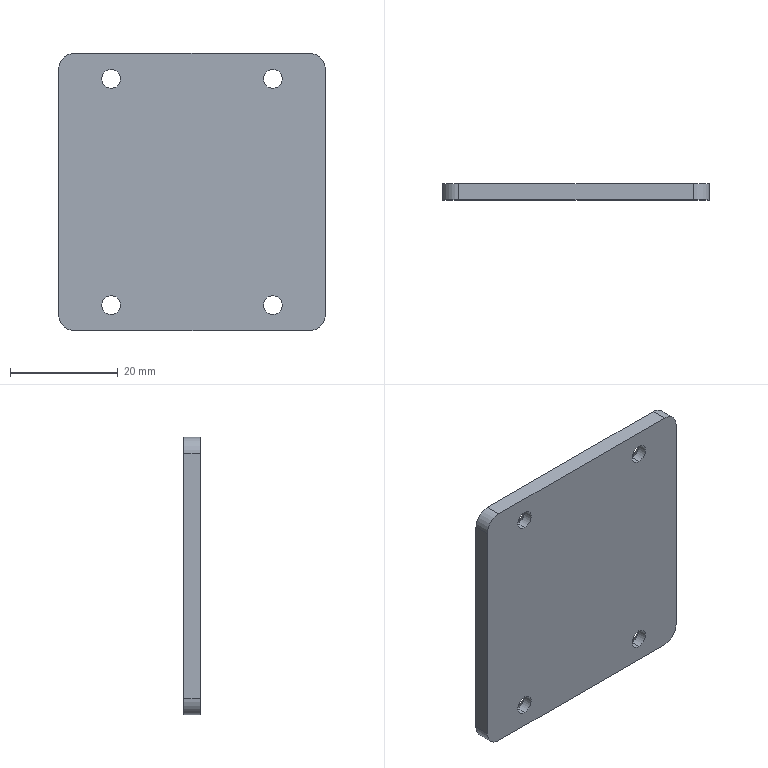Part | SolidWorks | features Chamfer 1, Extrusion 1, Fillet 1 | 1 solid | 26 faces | box 49.5 x 3 x 51.5 mm | volume 7470 mm3 | cylinder 12 | cone 8 | plane 6 | commonest cylinder face diameters 3.5 x8 6 x4
STEP:
#1=CARTESIAN_POINT('',(-15.,1.8,-22.75));
#2=VERTEX_POINT('',#1);
#3=CARTESIAN_POINT('',(-15.,1.8,-19.25));
#4=VERTEX_POINT('',#3);
#5=CARTESIAN_POINT('',(-15.,1.8,-21.));
#6=DIRECTION('',(0.,1.,0.));
#7=DIRECTION('',(0.,0.,1.));
#8=AXIS2_PLACEMENT_3D('',#5,#6,#7);
#9=CIRCLE('',#8,1.75);
#10=EDGE_CURVE('',#2,#4,#9,.T.);
#11=ORIENTED_EDGE('',*,*,#10,.F.);
#12=CARTESIAN_POINT('',(-15.,3.,-23.95));
#13=VERTEX_POINT('',#12);
#14=CARTESIAN_POINT('',(-15.,1.8,-22.75));
#15=DIRECTION('',(0.,0.7071,-0.7071));
#16=VECTOR('',#15,1000.);
#17=LINE('',#14,#16);
#18=EDGE_CURVE('',#2,#13,#17,.T.);
#19=ORIENTED_EDGE('',*,*,#18,.T.);
#20=CARTESIAN_POINT('',(-15.,3.,-18.05));
#21=VERTEX_POINT('',#20);
#22=CARTESIAN_POINT('',(-15.,3.,-21.));
#23=DIRECTION('',(0.,-1.,0.));
#24=DIRECTION('',(0.,0.,1.));
#25=AXIS2_PLACEMENT_3D('',#22,#23,#24);
#26=CIRCLE('',#25,2.95);
#27=EDGE_CURVE('',#21,#13,#26,.T.);
#28=ORIENTED_EDGE('',*,*,#27,.F.);
#29=CARTESIAN_POINT('',(-15.,1.8,-19.25));
#30=DIRECTION('',(0.,0.7071,0.7071));
#31=VECTOR('',#30,1000.);
#32=LINE('',#29,#31);
#33=EDGE_CURVE('',#4,#21,#32,.T.);
#34=ORIENTED_EDGE('',*,*,#33,.F.);
#35=EDGE_LOOP('',(#11,#19,#28,#34));
#36=FACE_OUTER_BOUND('',#35,.T.);
#37=CARTESIAN_POINT('',(-15.,1.8,-21.));
#38=DIRECTION('',(0.,1.,0.));
#39=DIRECTION('',(0.,0.,1.));
#40=AXIS2_PLACEMENT_3D('',#37,#38,#39);
#41=CONICAL_SURFACE('',#40,1.75,0.7854);
#42=ADVANCED_FACE('',(#36),#41,.F.);
#43=CARTESIAN_POINT('',(15.,1.8,-22.75));
#44=VERTEX_POINT('',#43);
#45=CARTESIAN_POINT('',(15.,1.8,-19.25));
#46=VERTEX_POINT('',#45);
#47=CARTESIAN_POINT('',(15.,1.8,-21.));
#48=DIRECTION('',(0.,1.,0.));
#49=DIRECTION('',(0.,0.,1.));
#50=AXIS2_PLACEMENT_3D('',#47,#48,#49);
#51=CIRCLE('',#50,1.75);
#52=EDGE_CURVE('',#44,#46,#51,.T.);
#53=ORIENTED_EDGE('',*,*,#52,.F.);
#54=CARTESIAN_POINT('',(15.,3.,-23.95));
#55=VERTEX_POINT('',#54);
#56=CARTESIAN_POINT('',(15.,1.8,-22.75));
#57=DIRECTION('',(0.,0.7071,-0.7071));
#58=VECTOR('',#57,1000.);
#59=LINE('',#56,#58);
#60=EDGE_CURVE('',#44,#55,#59,.T.);
#61=ORIENTED_EDGE('',*,*,#60,.T.);
#62=CARTESIAN_POINT('',(15.,3.,-18.05));
#63=VERTEX_POINT('',#62);
#64=CARTESIAN_POINT('',(15.,3.,-21.));
#65=DIRECTION('',(0.,-1.,0.));
#66=DIRECTION('',(0.,0.,1.));
#67=AXIS2_PLACEMENT_3D('',#64,#65,#66);
#68=CIRCLE('',#67,2.95);
#69=EDGE_CURVE('',#63,#55,#68,.T.);
#70=ORIENTED_EDGE('',*,*,#69,.F.);
#71=CARTESIAN_POINT('',(15.,1.8,-19.25));
#72=DIRECTION('',(0.,0.7071,0.7071));
#73=VECTOR('',#72,1000.);
#74=LINE('',#71,#73);
#75=EDGE_CURVE('',#46,#63,#74,.T.);
#76=ORIENTED_EDGE('',*,*,#75,.F.);
#77=EDGE_LOOP('',(#53,#61,#70,#76));
#78=FACE_OUTER_BOUND('',#77,.T.);
#79=CARTESIAN_POINT('',(15.,1.8,-21.));
#80=DIRECTION('',(0.,1.,0.));
#81=DIRECTION('',(0.,0.,1.));
#82=AXIS2_PLACEMENT_3D('',#79,#80,#81);
#83=CONICAL_SURFACE('',#82,1.75,0.7854);
#84=ADVANCED_FACE('',(#78),#83,.F.);
#85=CARTESIAN_POINT('',(15.,1.8,19.25));
#86=VERTEX_POINT('',#85);
#87=CARTESIAN_POINT('',(15.,1.8,22.75));
#88=VERTEX_POINT('',#87);
#89=CARTESIAN_POINT('',(15.,1.8,21.));
#90=DIRECTION('',(0.,1.,0.));
#91=DIRECTION('',(0.,0.,1.));
#92=AXIS2_PLACEMENT_3D('',#89,#90,#91);
#93=CIRCLE('',#92,1.75);
#94=EDGE_CURVE('',#86,#88,#93,.T.);
#95=ORIENTED_EDGE('',*,*,#94,.F.);
#96=CARTESIAN_POINT('',(15.,3.,18.05));
#97=VERTEX_POINT('',#96);
#98=CARTESIAN_POINT('',(15.,1.8,19.25));
#99=DIRECTION('',(0.,0.7071,-0.7071));
#100=VECTOR('',#99,1000.);
#101=LINE('',#98,#100);
#102=EDGE_CURVE('',#86,#97,#101,.T.);
#103=ORIENTED_EDGE('',*,*,#102,.T.);
#104=CARTESIAN_POINT('',(15.,3.,23.95));
#105=VERTEX_POINT('',#104);
#106=CARTESIAN_POINT('',(15.,3.,21.));
#107=DIRECTION('',(0.,-1.,0.));
#108=DIRECTION('',(0.,0.,1.));
#109=AXIS2_PLACEMENT_3D('',#106,#107,#108);
#110=CIRCLE('',#109,2.95);
#111=EDGE_CURVE('',#105,#97,#110,.T.);
#112=ORIENTED_EDGE('',*,*,#111,.F.);
#113=CARTESIAN_POINT('',(15.,1.8,22.75));
#114=DIRECTION('',(0.,0.7071,0.7071));
#115=VECTOR('',#114,1000.);
#116=LINE('',#113,#115);
#117=EDGE_CURVE('',#88,#105,#116,.T.);
#118=ORIENTED_EDGE('',*,*,#117,.F.);
#119=EDGE_LOOP('',(#95,#103,#112,#118));
#120=FACE_OUTER_BOUND('',#119,.T.);
#121=CARTESIAN_POINT('',(15.,1.8,21.));
#122=DIRECTION('',(0.,1.,0.));
#123=DIRECTION('',(0.,0.,1.));
#124=AXIS2_PLACEMENT_3D('',#121,#122,#123);
#125=CONICAL_SURFACE('',#124,1.75,0.7854);
#126=ADVANCED_FACE('',(#120),#125,.F.);
#127=CARTESIAN_POINT('',(-15.,1.8,19.25));
#128=VERTEX_POINT('',#127);
#129=CARTESIAN_POINT('',(-15.,1.8,22.75));
#130=VERTEX_POINT('',#129);
#131=CARTESIAN_POINT('',(-15.,1.8,21.));
#132=DIRECTION('',(0.,1.,0.));
#133=DIRECTION('',(0.,0.,1.));
#134=AXIS2_PLACEMENT_3D('',#131,#132,#133);
#135=CIRCLE('',#134,1.75);
#136=EDGE_CURVE('',#128,#130,#135,.T.);
#137=ORIENTED_EDGE('',*,*,#136,.F.);
#138=CARTESIAN_POINT('',(-15.,3.,18.05));
#139=VERTEX_POINT('',#138);
#140=CARTESIAN_POINT('',(-15.,1.8,19.25));
#141=DIRECTION('',(0.,0.7071,-0.7071));
#142=VECTOR('',#141,1000.);
#143=LINE('',#140,#142);
#144=EDGE_CURVE('',#128,#139,#143,.T.);
#145=ORIENTED_EDGE('',*,*,#144,.T.);
#146=CARTESIAN_POINT('',(-15.,3.,23.95));
#147=VERTEX_POINT('',#146);
#148=CARTESIAN_POINT('',(-15.,3.,21.));
#149=DIRECTION('',(0.,-1.,0.));
#150=DIRECTION('',(0.,0.,1.));
#151=AXIS2_PLACEMENT_3D('',#148,#149,#150);
#152=CIRCLE('',#151,2.95);
#153=EDGE_CURVE('',#147,#139,#152,.T.);
#154=ORIENTED_EDGE('',*,*,#153,.F.);
#155=CARTESIAN_POINT('',(-15.,1.8,22.75));
#156=DIRECTION('',(0.,0.7071,0.7071));
#157=VECTOR('',#156,1000.);
#158=LINE('',#155,#157);
#159=EDGE_CURVE('',#130,#147,#158,.T.);
#160=ORIENTED_EDGE('',*,*,#159,.F.);
#161=EDGE_LOOP('',(#137,#145,#154,#160));
#162=FACE_OUTER_BOUND('',#161,.T.);
#163=CARTESIAN_POINT('',(-15.,1.8,21.));
#164=DIRECTION('',(0.,1.,0.));
#165=DIRECTION('',(0.,0.,1.));
#166=AXIS2_PLACEMENT_3D('',#163,#164,#165);
#167=CONICAL_SURFACE('',#166,1.75,0.7854);
#168=ADVANCED_FACE('',(#162),#167,.F.);
#169=ORIENTED_EDGE('',*,*,#94,.T.);
#170=CARTESIAN_POINT('',(15.,0.,22.75));
#171=VERTEX_POINT('',#170);
#172=CARTESIAN_POINT('',(15.,3.,22.75));
#173=DIRECTION('',(0.,-1.,0.));
#174=VECTOR('',#173,1000.);
#175=LINE('',#172,#174);
#176=EDGE_CURVE('',#88,#171,#175,.T.);
#177=ORIENTED_EDGE('',*,*,#176,.T.);
#178=CARTESIAN_POINT('',(15.,0.,19.25));
#179=VERTEX_POINT('',#178);
#180=CARTESIAN_POINT('',(15.,0.,21.));
#181=DIRECTION('',(0.,1.,0.));
#182=DIRECTION('',(0.,0.,1.));
#183=AXIS2_PLACEMENT_3D('',#180,#181,#182);
#184=CIRCLE('',#183,1.75);
#185=EDGE_CURVE('',#179,#171,#184,.T.);
#186=ORIENTED_EDGE('',*,*,#185,.F.);
#187=CARTESIAN_POINT('',(15.,3.,19.25));
#188=DIRECTION('',(0.,-1.,0.));
#189=VECTOR('',#188,1000.);
#190=LINE('',#187,#189);
#191=EDGE_CURVE('',#86,#179,#190,.T.);
#192=ORIENTED_EDGE('',*,*,#191,.F.);
#193=EDGE_LOOP('',(#169,#177,#186,#192));
#194=FACE_OUTER_BOUND('',#193,.T.);
#195=CARTESIAN_POINT('',(15.,3.,21.));
#196=DIRECTION('',(0.,-1.,0.));
#197=DIRECTION('',(0.,0.,-1.));
#198=AXIS2_PLACEMENT_3D('',#195,#196,#197);
#199=CYLINDRICAL_SURFACE('',#198,1.75);
#200=ADVANCED_FACE('',(#194),#199,.F.);
#201=ORIENTED_EDGE('',*,*,#136,.T.);
#202=CARTESIAN_POINT('',(-15.,0.,22.75));
#203=VERTEX_POINT('',#202);
#204=CARTESIAN_POINT('',(-15.,3.,22.75));
#205=DIRECTION('',(0.,-1.,0.));
#206=VECTOR('',#205,1000.);
#207=LINE('',#204,#206);
#208=EDGE_CURVE('',#130,#203,#207,.T.);
#209=ORIENTED_EDGE('',*,*,#208,.T.);
#210=CARTESIAN_POINT('',(-15.,0.,19.25));
#211=VERTEX_POINT('',#210);
#212=CARTESIAN_POINT('',(-15.,0.,21.));
#213=DIRECTION('',(0.,1.,0.));
#214=DIRECTION('',(0.,0.,1.));
#215=AXIS2_PLACEMENT_3D('',#212,#213,#214);
#216=CIRCLE('',#215,1.75);
#217=EDGE_CURVE('',#211,#203,#216,.T.);
#218=ORIENTED_EDGE('',*,*,#217,.F.);
#219=CARTESIAN_POINT('',(-15.,3.,19.25));
#220=DIRECTION('',(0.,-1.,0.));
#221=VECTOR('',#220,1000.);
#222=LINE('',#219,#221);
#223=EDGE_CURVE('',#128,#211,#222,.T.);
#224=ORIENTED_EDGE('',*,*,#223,.F.);
#225=EDGE_LOOP('',(#201,#209,#218,#224));
#226=FACE_OUTER_BOUND('',#225,.T.);
#227=CARTESIAN_POINT('',(-15.,3.,21.));
#228=DIRECTION('',(0.,-1.,0.));
#229=DIRECTION('',(0.,0.,-1.));
#230=AXIS2_PLACEMENT_3D('',#227,#228,#229);
#231=CYLINDRICAL_SURFACE('',#230,1.75);
#232=ADVANCED_FACE('',(#226),#231,.F.);
#233=ORIENTED_EDGE('',*,*,#52,.T.);
#234=CARTESIAN_POINT('',(15.,0.,-19.25));
#235=VERTEX_POINT('',#234);
#236=CARTESIAN_POINT('',(15.,3.,-19.25));
#237=DIRECTION('',(0.,-1.,0.));
#238=VECTOR('',#237,1000.);
#239=LINE('',#236,#238);
#240=EDGE_CURVE('',#46,#235,#239,.T.);
#241=ORIENTED_EDGE('',*,*,#240,.T.);
#242=CARTESIAN_POINT('',(15.,0.,-22.75));
#243=VERTEX_POINT('',#242);
#244=CARTESIAN_POINT('',(15.,0.,-21.));
#245=DIRECTION('',(0.,1.,0.));
#246=DIRECTION('',(0.,0.,1.));
#247=AXIS2_PLACEMENT_3D('',#244,#245,#246);
#248=CIRCLE('',#247,1.75);
#249=EDGE_CURVE('',#243,#235,#248,.T.);
#250=ORIENTED_EDGE('',*,*,#249,.F.);
#251=CARTESIAN_POINT('',(15.,3.,-22.75));
#252=DIRECTION('',(0.,-1.,0.));
#253=VECTOR('',#252,1000.);
#254=LINE('',#251,#253);
#255=EDGE_CURVE('',#44,#243,#254,.T.);
#256=ORIENTED_EDGE('',*,*,#255,.F.);
#257=EDGE_LOOP('',(#233,#241,#250,#256));
#258=FACE_OUTER_BOUND('',#257,.T.);
#259=CARTESIAN_POINT('',(15.,3.,-21.));
#260=DIRECTION('',(0.,-1.,0.));
#261=DIRECTION('',(0.,0.,-1.));
#262=AXIS2_PLACEMENT_3D('',#259,#260,#261);
#263=CYLINDRICAL_SURFACE('',#262,1.75);
#264=ADVANCED_FACE('',(#258),#263,.F.);
#265=ORIENTED_EDGE('',*,*,#10,.T.);
#266=CARTESIAN_POINT('',(-15.,0.,-19.25));
#267=VERTEX_POINT('',#266);
#268=CARTESIAN_POINT('',(-15.,3.,-19.25));
#269=DIRECTION('',(0.,-1.,0.));
#270=VECTOR('',#269,1000.);
#271=LINE('',#268,#270);
#272=EDGE_CURVE('',#4,#267,#271,.T.);
#273=ORIENTED_EDGE('',*,*,#272,.T.);
#274=CARTESIAN_POINT('',(-15.,0.,-22.75));
#275=VERTEX_POINT('',#274);
#276=CARTESIAN_POINT('',(-15.,0.,-21.));
#277=DIRECTION('',(0.,1.,0.));
#278=DIRECTION('',(0.,0.,1.));
#279=AXIS2_PLACEMENT_3D('',#276,#277,#278);
#280=CIRCLE('',#279,1.75);
#281=EDGE_CURVE('',#275,#267,#280,.T.);
#282=ORIENTED_EDGE('',*,*,#281,.F.);
#283=CARTESIAN_POINT('',(-15.,3.,-22.75));
#284=DIRECTION('',(0.,-1.,0.));
#285=VECTOR('',#284,1000.);
#286=LINE('',#283,#285);
#287=EDGE_CURVE('',#2,#275,#286,.T.);
#288=ORIENTED_EDGE('',*,*,#287,.F.);
#289=EDGE_LOOP('',(#265,#273,#282,#288));
#290=FACE_OUTER_BOUND('',#289,.T.);
#291=CARTESIAN_POINT('',(-15.,3.,-21.));
#292=DIRECTION('',(0.,-1.,0.));
#293=DIRECTION('',(0.,0.,-1.));
#294=AXIS2_PLACEMENT_3D('',#291,#292,#293);
#295=CYLINDRICAL_SURFACE('',#294,1.75);
#296=ADVANCED_FACE('',(#290),#295,.F.);
#297=ORIENTED_EDGE('',*,*,#153,.T.);
#298=CARTESIAN_POINT('',(-15.,3.,21.));
#299=DIRECTION('',(0.,-1.,0.));
#300=DIRECTION('',(0.,0.,1.));
#301=AXIS2_PLACEMENT_3D('',#298,#299,#300);
#302=CIRCLE('',#301,2.95);
#303=EDGE_CURVE('',#139,#147,#302,.T.);
#304=ORIENTED_EDGE('',*,*,#303,.T.);
#305=EDGE_LOOP('',(#297,#304));
#306=FACE_BOUND('',#305,.T.);
#307=ORIENTED_EDGE('',*,*,#111,.T.);
#308=CARTESIAN_POINT('',(15.,3.,21.));
#309=DIRECTION('',(0.,-1.,0.));
#310=DIRECTION('',(0.,0.,1.));
#311=AXIS2_PLACEMENT_3D('',#308,#309,#310);
#312=CIRCLE('',#311,2.95);
#313=EDGE_CURVE('',#97,#105,#312,.T.);
#314=ORIENTED_EDGE('',*,*,#313,.T.);
#315=EDGE_LOOP('',(#307,#314));
#316=FACE_BOUND('',#315,.T.);
#317=ORIENTED_EDGE('',*,*,#69,.T.);
#318=CARTESIAN_POINT('',(15.,3.,-21.));
#319=DIRECTION('',(0.,-1.,0.));
#320=DIRECTION('',(0.,0.,1.));
#321=AXIS2_PLACEMENT_3D('',#318,#319,#320);
#322=CIRCLE('',#321,2.95);
#323=EDGE_CURVE('',#55,#63,#322,.T.);
#324=ORIENTED_EDGE('',*,*,#323,.T.);
#325=EDGE_LOOP('',(#317,#324));
#326=FACE_BOUND('',#325,.T.);
#327=ORIENTED_EDGE('',*,*,#27,.T.);
#328=CARTESIAN_POINT('',(-15.,3.,-21.));
#329=DIRECTION('',(0.,-1.,0.));
#330=DIRECTION('',(0.,0.,1.));
#331=AXIS2_PLACEMENT_3D('',#328,#329,#330);
#332=CIRCLE('',#331,2.95);
#333=EDGE_CURVE('',#13,#21,#332,.T.);
#334=ORIENTED_EDGE('',*,*,#333,.T.);
#335=EDGE_LOOP('',(#327,#334));
#336=FACE_BOUND('',#335,.T.);
#337=CARTESIAN_POINT('',(-24.75,3.,-22.75));
#338=VERTEX_POINT('',#337);
#339=CARTESIAN_POINT('',(-24.75,3.,22.75));
#340=VERTEX_POINT('',#339);
#341=CARTESIAN_POINT('',(-24.75,3.,-25.75));
#342=DIRECTION('',(0.,0.,1.));
#343=VECTOR('',#342,1000.);
#344=LINE('',#341,#343);
#345=EDGE_CURVE('',#338,#340,#344,.T.);
#346=ORIENTED_EDGE('',*,*,#345,.T.);
#347=CARTESIAN_POINT('',(-21.75,3.,25.75));
#348=VERTEX_POINT('',#347);
#349=CARTESIAN_POINT('',(-21.75,3.,22.75));
#350=DIRECTION('',(0.,1.,0.));
#351=DIRECTION('',(0.,0.,1.));
#352=AXIS2_PLACEMENT_3D('',#349,#350,#351);
#353=CIRCLE('',#352,3.);
#354=EDGE_CURVE('',#340,#348,#353,.T.);
#355=ORIENTED_EDGE('',*,*,#354,.T.);
#356=CARTESIAN_POINT('',(21.75,3.,25.75));
#357=VERTEX_POINT('',#356);
#358=CARTESIAN_POINT('',(-24.75,3.,25.75));
#359=DIRECTION('',(1.,0.,0.));
#360=VECTOR('',#359,1000.);
#361=LINE('',#358,#360);
#362=EDGE_CURVE('',#348,#357,#361,.T.);
#363=ORIENTED_EDGE('',*,*,#362,.T.);
#364=CARTESIAN_POINT('',(24.75,3.,22.75));
#365=VERTEX_POINT('',#364);
#366=CARTESIAN_POINT('',(21.75,3.,22.75));
#367=DIRECTION('',(0.,1.,0.));
#368=DIRECTION('',(0.,0.,1.));
#369=AXIS2_PLACEMENT_3D('',#366,#367,#368);
#370=CIRCLE('',#369,3.);
#371=EDGE_CURVE('',#357,#365,#370,.T.);
#372=ORIENTED_EDGE('',*,*,#371,.T.);
#373=CARTESIAN_POINT('',(24.75,3.,-22.75));
#374=VERTEX_POINT('',#373);
#375=CARTESIAN_POINT('',(24.75,3.,-25.75));
#376=DIRECTION('',(0.,0.,-1.));
#377=VECTOR('',#376,1000.);
#378=LINE('',#375,#377);
#379=EDGE_CURVE('',#365,#374,#378,.T.);
#380=ORIENTED_EDGE('',*,*,#379,.T.);
#381=CARTESIAN_POINT('',(21.75,3.,-25.75));
#382=VERTEX_POINT('',#381);
#383=CARTESIAN_POINT('',(21.75,3.,-22.75));
#384=DIRECTION('',(0.,1.,0.));
#385=DIRECTION('',(0.,0.,1.));
#386=AXIS2_PLACEMENT_3D('',#383,#384,#385);
#387=CIRCLE('',#386,3.);
#388=EDGE_CURVE('',#374,#382,#387,.T.);
#389=ORIENTED_EDGE('',*,*,#388,.T.);
#390=CARTESIAN_POINT('',(-21.75,3.,-25.75));
#391=VERTEX_POINT('',#390);
#392=CARTESIAN_POINT('',(-24.75,3.,-25.75));
#393=DIRECTION('',(-1.,0.,0.));
#394=VECTOR('',#393,1000.);
#395=LINE('',#392,#394);
#396=EDGE_CURVE('',#382,#391,#395,.T.);
#397=ORIENTED_EDGE('',*,*,#396,.T.);
#398=CARTESIAN_POINT('',(-21.75,3.,-22.75));
#399=DIRECTION('',(0.,1.,0.));
#400=DIRECTION('',(0.,0.,1.));
#401=AXIS2_PLACEMENT_3D('',#398,#399,#400);
#402=CIRCLE('',#401,3.);
#403=EDGE_CURVE('',#391,#338,#402,.T.);
#404=ORIENTED_EDGE('',*,*,#403,.T.);
#405=EDGE_LOOP('',(#346,#355,#363,#372,#380,#389,#397,#404));
#406=FACE_OUTER_BOUND('',#405,.T.);
#407=CARTESIAN_POINT('',(0.,3.,0.));
#408=DIRECTION('',(0.,1.,0.));
#409=DIRECTION('',(0.,0.,1.));
#410=AXIS2_PLACEMENT_3D('',#407,#408,#409);
#411=PLANE('',#410);
#412=ADVANCED_FACE('',(#306,#316,#326,#336,#406),#411,.T.);
#413=CARTESIAN_POINT('',(-21.75,0.,25.75));
#414=VERTEX_POINT('',#413);
#415=CARTESIAN_POINT('',(21.75,0.,25.75));
#416=VERTEX_POINT('',#415);
#417=CARTESIAN_POINT('',(-24.75,0.,25.75));
#418=DIRECTION('',(1.,0.,0.));
#419=VECTOR('',#418,1000.);
#420=LINE('',#417,#419);
#421=EDGE_CURVE('',#414,#416,#420,.T.);
#422=ORIENTED_EDGE('',*,*,#421,.F.);
#423=CARTESIAN_POINT('',(-24.75,0.,22.75));
#424=VERTEX_POINT('',#423);
#425=CARTESIAN_POINT('',(-21.75,0.,22.75));
#426=DIRECTION('',(0.,-1.,0.));
#427=DIRECTION('',(0.,0.,1.));
#428=AXIS2_PLACEMENT_3D('',#425,#426,#427);
#429=CIRCLE('',#428,3.);
#430=EDGE_CURVE('',#414,#424,#429,.T.);
#431=ORIENTED_EDGE('',*,*,#430,.T.);
#432=CARTESIAN_POINT('',(-24.75,0.,-22.75));
#433=VERTEX_POINT('',#432);
#434=CARTESIAN_POINT('',(-24.75,0.,-25.75));
#435=DIRECTION('',(0.,0.,1.));
#436=VECTOR('',#435,1000.);
#437=LINE('',#434,#436);
#438=EDGE_CURVE('',#433,#424,#437,.T.);
#439=ORIENTED_EDGE('',*,*,#438,.F.);
#440=CARTESIAN_POINT('',(-21.75,0.,-25.75));
#441=VERTEX_POINT('',#440);
#442=CARTESIAN_POINT('',(-21.75,0.,-22.75));
#443=DIRECTION('',(0.,-1.,0.));
#444=DIRECTION('',(0.,0.,1.));
#445=AXIS2_PLACEMENT_3D('',#442,#443,#444);
#446=CIRCLE('',#445,3.);
#447=EDGE_CURVE('',#433,#441,#446,.T.);
#448=ORIENTED_EDGE('',*,*,#447,.T.);
#449=CARTESIAN_POINT('',(21.75,0.,-25.75));
#450=VERTEX_POINT('',#449);
#451=CARTESIAN_POINT('',(-24.75,0.,-25.75));
#452=DIRECTION('',(-1.,0.,0.));
#453=VECTOR('',#452,1000.);
#454=LINE('',#451,#453);
#455=EDGE_CURVE('',#450,#441,#454,.T.);
#456=ORIENTED_EDGE('',*,*,#455,.F.);
#457=CARTESIAN_POINT('',(24.75,0.,-22.75));
#458=VERTEX_POINT('',#457);
#459=CARTESIAN_POINT('',(21.75,0.,-22.75));
#460=DIRECTION('',(0.,-1.,0.));
#461=DIRECTION('',(0.,0.,1.));
#462=AXIS2_PLACEMENT_3D('',#459,#460,#461);
#463=CIRCLE('',#462,3.);
#464=EDGE_CURVE('',#450,#458,#463,.T.);
#465=ORIENTED_EDGE('',*,*,#464,.T.);
#466=CARTESIAN_POINT('',(24.75,0.,22.75));
#467=VERTEX_POINT('',#466);
#468=CARTESIAN_POINT('',(24.75,0.,-25.75));
#469=DIRECTION('',(0.,0.,-1.));
#470=VECTOR('',#469,1000.);
#471=LINE('',#468,#470);
#472=EDGE_CURVE('',#467,#458,#471,.T.);
#473=ORIENTED_EDGE('',*,*,#472,.F.);
#474=CARTESIAN_POINT('',(21.75,0.,22.75));
#475=DIRECTION('',(0.,-1.,0.));
#476=DIRECTION('',(0.,0.,1.));
#477=AXIS2_PLACEMENT_3D('',#474,#475,#476);
#478=CIRCLE('',#477,3.);
#479=EDGE_CURVE('',#467,#416,#478,.T.);
#480=ORIENTED_EDGE('',*,*,#479,.T.);
#481=EDGE_LOOP('',(#422,#431,#439,#448,#456,#465,#473,#480));
#482=FACE_OUTER_BOUND('',#481,.T.);
#483=ORIENTED_EDGE('',*,*,#281,.T.);
#484=CARTESIAN_POINT('',(-15.,0.,-21.));
#485=DIRECTION('',(0.,1.,0.));
#486=DIRECTION('',(0.,0.,1.));
#487=AXIS2_PLACEMENT_3D('',#484,#485,#486);
#488=CIRCLE('',#487,1.75);
#489=EDGE_CURVE('',#267,#275,#488,.T.);
#490=ORIENTED_EDGE('',*,*,#489,.T.);
#491=EDGE_LOOP('',(#483,#490));
#492=FACE_BOUND('',#491,.T.);
#493=ORIENTED_EDGE('',*,*,#249,.T.);
#494=CARTESIAN_POINT('',(15.,0.,-21.));
#495=DIRECTION('',(0.,1.,0.));
#496=DIRECTION('',(0.,0.,1.));
#497=AXIS2_PLACEMENT_3D('',#494,#495,#496);
#498=CIRCLE('',#497,1.75);
#499=EDGE_CURVE('',#235,#243,#498,.T.);
#500=ORIENTED_EDGE('',*,*,#499,.T.);
#501=EDGE_LOOP('',(#493,#500));
#502=FACE_BOUND('',#501,.T.);
#503=ORIENTED_EDGE('',*,*,#217,.T.);
#504=CARTESIAN_POINT('',(-15.,0.,21.));
#505=DIRECTION('',(0.,1.,0.));
#506=DIRECTION('',(0.,0.,1.));
#507=AXIS2_PLACEMENT_3D('',#504,#505,#506);
#508=CIRCLE('',#507,1.75);
#509=EDGE_CURVE('',#203,#211,#508,.T.);
#510=ORIENTED_EDGE('',*,*,#509,.T.);
#511=EDGE_LOOP('',(#503,#510));
#512=FACE_BOUND('',#511,.T.);
#513=ORIENTED_EDGE('',*,*,#185,.T.);
#514=CARTESIAN_POINT('',(15.,0.,21.));
#515=DIRECTION('',(0.,1.,0.));
#516=DIRECTION('',(0.,0.,1.));
#517=AXIS2_PLACEMENT_3D('',#514,#515,#516);
#518=CIRCLE('',#517,1.75);
#519=EDGE_CURVE('',#171,#179,#518,.T.);
#520=ORIENTED_EDGE('',*,*,#519,.T.);
#521=EDGE_LOOP('',(#513,#520));
#522=FACE_BOUND('',#521,.T.);
#523=CARTESIAN_POINT('',(0.,0.,0.));
#524=DIRECTION('',(0.,1.,0.));
#525=DIRECTION('',(0.,0.,1.));
#526=AXIS2_PLACEMENT_3D('',#523,#524,#525);
#527=PLANE('',#526);
#528=ADVANCED_FACE('',(#482,#492,#502,#512,#522),#527,.F.);
#529=ORIENTED_EDGE('',*,*,#472,.T.);
#530=CARTESIAN_POINT('',(24.75,3.,-22.75));
#531=DIRECTION('',(0.,1.,0.));
#532=VECTOR('',#531,1000.);
#533=LINE('',#530,#532);
#534=EDGE_CURVE('',#458,#374,#533,.T.);
#535=ORIENTED_EDGE('',*,*,#534,.T.);
#536=ORIENTED_EDGE('',*,*,#379,.F.);
#537=CARTESIAN_POINT('',(24.75,3.,22.75));
#538=DIRECTION('',(0.,-1.,0.));
#539=VECTOR('',#538,1000.);
#540=LINE('',#537,#539);
#541=EDGE_CURVE('',#365,#467,#540,.T.);
#542=ORIENTED_EDGE('',*,*,#541,.T.);
#543=EDGE_LOOP('',(#529,#535,#536,#542));
#544=FACE_OUTER_BOUND('',#543,.T.);
#545=CARTESIAN_POINT('',(24.75,3.,-25.75));
#546=DIRECTION('',(-1.,0.,0.));
#547=DIRECTION('',(0.,0.,1.));
#548=AXIS2_PLACEMENT_3D('',#545,#546,#547);
#549=PLANE('',#548);
#550=ADVANCED_FACE('',(#544),#549,.F.);
#551=ORIENTED_EDGE('',*,*,#455,.T.);
#552=CARTESIAN_POINT('',(-21.75,3.,-25.75));
#553=DIRECTION('',(0.,1.,0.));
#554=VECTOR('',#553,1000.);
#555=LINE('',#552,#554);
#556=EDGE_CURVE('',#441,#391,#555,.T.);
#557=ORIENTED_EDGE('',*,*,#556,.T.);
#558=ORIENTED_EDGE('',*,*,#396,.F.);
#559=CARTESIAN_POINT('',(21.75,3.,-25.75));
#560=DIRECTION('',(0.,-1.,0.));
#561=VECTOR('',#560,1000.);
#562=LINE('',#559,#561);
#563=EDGE_CURVE('',#382,#450,#562,.T.);
#564=ORIENTED_EDGE('',*,*,#563,.T.);
#565=EDGE_LOOP('',(#551,#557,#558,#564));
#566=FACE_OUTER_BOUND('',#565,.T.);
#567=CARTESIAN_POINT('',(-24.75,3.,-25.75));
#568=DIRECTION('',(0.,0.,1.));
#569=DIRECTION('',(1.,0.,0.));
#570=AXIS2_PLACEMENT_3D('',#567,#568,#569);
#571=PLANE('',#570);
#572=ADVANCED_FACE('',(#566),#571,.F.);
#573=ORIENTED_EDGE('',*,*,#438,.T.);
#574=CARTESIAN_POINT('',(-24.75,3.,22.75));
#575=DIRECTION('',(0.,1.,0.));
#576=VECTOR('',#575,1000.);
#577=LINE('',#574,#576);
#578=EDGE_CURVE('',#424,#340,#577,.T.);
#579=ORIENTED_EDGE('',*,*,#578,.T.);
#580=ORIENTED_EDGE('',*,*,#345,.F.);
#581=CARTESIAN_POINT('',(-24.75,3.,-22.75));
#582=DIRECTION('',(0.,-1.,0.));
#583=VECTOR('',#582,1000.);
#584=LINE('',#581,#583);
#585=EDGE_CURVE('',#338,#433,#584,.T.);
#586=ORIENTED_EDGE('',*,*,#585,.T.);
#587=EDGE_LOOP('',(#573,#579,#580,#586));
#588=FACE_OUTER_BOUND('',#587,.T.);
#589=CARTESIAN_POINT('',(-24.75,3.,-25.75));
#590=DIRECTION('',(1.,0.,0.));
#591=DIRECTION('',(0.,0.,-1.));
#592=AXIS2_PLACEMENT_3D('',#589,#590,#591);
#593=PLANE('',#592);
#594=ADVANCED_FACE('',(#588),#593,.F.);
#595=ORIENTED_EDGE('',*,*,#362,.F.);
#596=CARTESIAN_POINT('',(-21.75,3.,25.75));
#597=DIRECTION('',(0.,-1.,0.));
#598=VECTOR('',#597,1000.);
#599=LINE('',#596,#598);
#600=EDGE_CURVE('',#348,#414,#599,.T.);
#601=ORIENTED_EDGE('',*,*,#600,.T.);
#602=ORIENTED_EDGE('',*,*,#421,.T.);
#603=CARTESIAN_POINT('',(21.75,3.,25.75));
#604=DIRECTION('',(0.,1.,0.));
#605=VECTOR('',#604,1000.);
#606=LINE('',#603,#605);
#607=EDGE_CURVE('',#416,#357,#606,.T.);
#608=ORIENTED_EDGE('',*,*,#607,.T.);
#609=EDGE_LOOP('',(#595,#601,#602,#608));
#610=FACE_OUTER_BOUND('',#609,.T.);
#611=CARTESIAN_POINT('',(-24.75,3.,25.75));
#612=DIRECTION('',(0.,0.,-1.));
#613=DIRECTION('',(-1.,0.,0.));
#614=AXIS2_PLACEMENT_3D('',#611,#612,#613);
#615=PLANE('',#614);
#616=ADVANCED_FACE('',(#610),#615,.F.);
#617=ORIENTED_EDGE('',*,*,#272,.F.);
#618=CARTESIAN_POINT('',(-15.,1.8,-21.));
#619=DIRECTION('',(0.,1.,0.));
#620=DIRECTION('',(0.,0.,1.));
#621=AXIS2_PLACEMENT_3D('',#618,#619,#620);
#622=CIRCLE('',#621,1.75);
#623=EDGE_CURVE('',#4,#2,#622,.T.);
#624=ORIENTED_EDGE('',*,*,#623,.T.);
#625=ORIENTED_EDGE('',*,*,#287,.T.);
#626=ORIENTED_EDGE('',*,*,#489,.F.);
#627=EDGE_LOOP('',(#617,#624,#625,#626));
#628=FACE_OUTER_BOUND('',#627,.T.);
#629=CARTESIAN_POINT('',(-15.,3.,-21.));
#630=DIRECTION('',(0.,-1.,0.));
#631=DIRECTION('',(0.,0.,-1.));
#632=AXIS2_PLACEMENT_3D('',#629,#630,#631);
#633=CYLINDRICAL_SURFACE('',#632,1.75);
#634=ADVANCED_FACE('',(#628),#633,.F.);
#635=ORIENTED_EDGE('',*,*,#240,.F.);
#636=CARTESIAN_POINT('',(15.,1.8,-21.));
#637=DIRECTION('',(0.,1.,0.));
#638=DIRECTION('',(0.,0.,1.));
#639=AXIS2_PLACEMENT_3D('',#636,#637,#638);
#640=CIRCLE('',#639,1.75);
#641=EDGE_CURVE('',#46,#44,#640,.T.);
#642=ORIENTED_EDGE('',*,*,#641,.T.);
#643=ORIENTED_EDGE('',*,*,#255,.T.);
#644=ORIENTED_EDGE('',*,*,#499,.F.);
#645=EDGE_LOOP('',(#635,#642,#643,#644));
#646=FACE_OUTER_BOUND('',#645,.T.);
#647=CARTESIAN_POINT('',(15.,3.,-21.));
#648=DIRECTION('',(0.,-1.,0.));
#649=DIRECTION('',(0.,0.,-1.));
#650=AXIS2_PLACEMENT_3D('',#647,#648,#649);
#651=CYLINDRICAL_SURFACE('',#650,1.75);
#652=ADVANCED_FACE('',(#646),#651,.F.);
#653=ORIENTED_EDGE('',*,*,#208,.F.);
#654=CARTESIAN_POINT('',(-15.,1.8,21.));
#655=DIRECTION('',(0.,1.,0.));
#656=DIRECTION('',(0.,0.,1.));
#657=AXIS2_PLACEMENT_3D('',#654,#655,#656);
#658=CIRCLE('',#657,1.75);
#659=EDGE_CURVE('',#130,#128,#658,.T.);
#660=ORIENTED_EDGE('',*,*,#659,.T.);
#661=ORIENTED_EDGE('',*,*,#223,.T.);
#662=ORIENTED_EDGE('',*,*,#509,.F.);
#663=EDGE_LOOP('',(#653,#660,#661,#662));
#664=FACE_OUTER_BOUND('',#663,.T.);
#665=CARTESIAN_POINT('',(-15.,3.,21.));
#666=DIRECTION('',(0.,-1.,0.));
#667=DIRECTION('',(0.,0.,-1.));
#668=AXIS2_PLACEMENT_3D('',#665,#666,#667);
#669=CYLINDRICAL_SURFACE('',#668,1.75);
#670=ADVANCED_FACE('',(#664),#669,.F.);
#671=ORIENTED_EDGE('',*,*,#176,.F.);
#672=CARTESIAN_POINT('',(15.,1.8,21.));
#673=DIRECTION('',(0.,1.,0.));
#674=DIRECTION('',(0.,0.,1.));
#675=AXIS2_PLACEMENT_3D('',#672,#673,#674);
#676=CIRCLE('',#675,1.75);
#677=EDGE_CURVE('',#88,#86,#676,.T.);
#678=ORIENTED_EDGE('',*,*,#677,.T.);
#679=ORIENTED_EDGE('',*,*,#191,.T.);
#680=ORIENTED_EDGE('',*,*,#519,.F.);
#681=EDGE_LOOP('',(#671,#678,#679,#680));
#682=FACE_OUTER_BOUND('',#681,.T.);
#683=CARTESIAN_POINT('',(15.,3.,21.));
#684=DIRECTION('',(0.,-1.,0.));
#685=DIRECTION('',(0.,0.,-1.));
#686=AXIS2_PLACEMENT_3D('',#683,#684,#685);
#687=CYLINDRICAL_SURFACE('',#686,1.75);
#688=ADVANCED_FACE('',(#682),#687,.F.);
#689=ORIENTED_EDGE('',*,*,#144,.F.);
#690=ORIENTED_EDGE('',*,*,#659,.F.);
#691=ORIENTED_EDGE('',*,*,#159,.T.);
#692=ORIENTED_EDGE('',*,*,#303,.F.);
#693=EDGE_LOOP('',(#689,#690,#691,#692));
#694=FACE_OUTER_BOUND('',#693,.T.);
#695=CARTESIAN_POINT('',(-15.,1.8,21.));
#696=DIRECTION('',(0.,1.,0.));
#697=DIRECTION('',(0.,0.,1.));
#698=AXIS2_PLACEMENT_3D('',#695,#696,#697);
#699=CONICAL_SURFACE('',#698,1.75,0.7854);
#700=ADVANCED_FACE('',(#694),#699,.F.);
#701=ORIENTED_EDGE('',*,*,#102,.F.);
#702=ORIENTED_EDGE('',*,*,#677,.F.);
#703=ORIENTED_EDGE('',*,*,#117,.T.);
#704=ORIENTED_EDGE('',*,*,#313,.F.);
#705=EDGE_LOOP('',(#701,#702,#703,#704));
#706=FACE_OUTER_BOUND('',#705,.T.);
#707=CARTESIAN_POINT('',(15.,1.8,21.));
#708=DIRECTION('',(0.,1.,0.));
#709=DIRECTION('',(0.,0.,1.));
#710=AXIS2_PLACEMENT_3D('',#707,#708,#709);
#711=CONICAL_SURFACE('',#710,1.75,0.7854);
#712=ADVANCED_FACE('',(#706),#711,.F.);
#713=ORIENTED_EDGE('',*,*,#60,.F.);
#714=ORIENTED_EDGE('',*,*,#641,.F.);
#715=ORIENTED_EDGE('',*,*,#75,.T.);
#716=ORIENTED_EDGE('',*,*,#323,.F.);
#717=EDGE_LOOP('',(#713,#714,#715,#716));
#718=FACE_OUTER_BOUND('',#717,.T.);
#719=CARTESIAN_POINT('',(15.,1.8,-21.));
#720=DIRECTION('',(0.,1.,0.));
#721=DIRECTION('',(0.,0.,1.));
#722=AXIS2_PLACEMENT_3D('',#719,#720,#721);
#723=CONICAL_SURFACE('',#722,1.75,0.7854);
#724=ADVANCED_FACE('',(#718),#723,.F.);
#725=ORIENTED_EDGE('',*,*,#18,.F.);
#726=ORIENTED_EDGE('',*,*,#623,.F.);
#727=ORIENTED_EDGE('',*,*,#33,.T.);
#728=ORIENTED_EDGE('',*,*,#333,.F.);
#729=EDGE_LOOP('',(#725,#726,#727,#728));
#730=FACE_OUTER_BOUND('',#729,.T.);
#731=CARTESIAN_POINT('',(-15.,1.8,-21.));
#732=DIRECTION('',(0.,1.,0.));
#733=DIRECTION('',(0.,0.,1.));
#734=AXIS2_PLACEMENT_3D('',#731,#732,#733);
#735=CONICAL_SURFACE('',#734,1.75,0.7854);
#736=ADVANCED_FACE('',(#730),#735,.F.);
#737=ORIENTED_EDGE('',*,*,#354,.F.);
#738=ORIENTED_EDGE('',*,*,#578,.F.);
#739=ORIENTED_EDGE('',*,*,#430,.F.);
#740=ORIENTED_EDGE('',*,*,#600,.F.);
#741=EDGE_LOOP('',(#737,#738,#739,#740));
#742=FACE_OUTER_BOUND('',#741,.T.);
#743=CARTESIAN_POINT('',(-21.75,3.,22.75));
#744=DIRECTION('',(0.,-1.,0.));
#745=DIRECTION('',(0.,0.,-1.));
#746=AXIS2_PLACEMENT_3D('',#743,#744,#745);
#747=CYLINDRICAL_SURFACE('',#746,3.);
#748=ADVANCED_FACE('',(#742),#747,.T.);
#749=ORIENTED_EDGE('',*,*,#403,.F.);
#750=ORIENTED_EDGE('',*,*,#556,.F.);
#751=ORIENTED_EDGE('',*,*,#447,.F.);
#752=ORIENTED_EDGE('',*,*,#585,.F.);
#753=EDGE_LOOP('',(#749,#750,#751,#752));
#754=FACE_OUTER_BOUND('',#753,.T.);
#755=CARTESIAN_POINT('',(-21.75,3.,-22.75));
#756=DIRECTION('',(0.,-1.,0.));
#757=DIRECTION('',(0.,0.,-1.));
#758=AXIS2_PLACEMENT_3D('',#755,#756,#757);
#759=CYLINDRICAL_SURFACE('',#758,3.);
#760=ADVANCED_FACE('',(#754),#759,.T.);
#761=ORIENTED_EDGE('',*,*,#388,.F.);
#762=ORIENTED_EDGE('',*,*,#534,.F.);
#763=ORIENTED_EDGE('',*,*,#464,.F.);
#764=ORIENTED_EDGE('',*,*,#563,.F.);
#765=EDGE_LOOP('',(#761,#762,#763,#764));
#766=FACE_OUTER_BOUND('',#765,.T.);
#767=CARTESIAN_POINT('',(21.75,3.,-22.75));
#768=DIRECTION('',(0.,-1.,0.));
#769=DIRECTION('',(0.,0.,-1.));
#770=AXIS2_PLACEMENT_3D('',#767,#768,#769);
#771=CYLINDRICAL_SURFACE('',#770,3.);
#772=ADVANCED_FACE('',(#766),#771,.T.);
#773=ORIENTED_EDGE('',*,*,#371,.F.);
#774=ORIENTED_EDGE('',*,*,#607,.F.);
#775=ORIENTED_EDGE('',*,*,#479,.F.);
#776=ORIENTED_EDGE('',*,*,#541,.F.);
#777=EDGE_LOOP('',(#773,#774,#775,#776));
#778=FACE_OUTER_BOUND('',#777,.T.);
#779=CARTESIAN_POINT('',(21.75,3.,22.75));
#780=DIRECTION('',(0.,-1.,0.));
#781=DIRECTION('',(0.,0.,-1.));
#782=AXIS2_PLACEMENT_3D('',#779,#780,#781);
#783=CYLINDRICAL_SURFACE('',#782,3.);
#784=ADVANCED_FACE('',(#778),#783,.T.);
#785=CLOSED_SHELL('',(#42,#84,#126,#168,#200,#232,#264,#296,#412,#528,#550,#572,#594,#616,#634,#652,#670,#688,#700,#712,#724,#736,#748,#760,#772,#784));
#786=MANIFOLD_SOLID_BREP('',#785);
#787=CARTESIAN_POINT('',(0.,0.,0.));
#788=DIRECTION('',(0.,0.,1.));
#789=DIRECTION('',(1.,0.,0.));
#790=AXIS2_PLACEMENT_3D('',#787,#788,#789);
#791=(LENGTH_UNIT()NAMED_UNIT(*)SI_UNIT(.MILLI.,.METRE.));
#792=UNCERTAINTY_MEASURE_WITH_UNIT(LENGTH_MEASURE(0.00001),#791,'','');
#793=(NAMED_UNIT(*)PLANE_ANGLE_UNIT()SI_UNIT($,.RADIAN.));
#794=(NAMED_UNIT(*)SI_UNIT($,.STERADIAN.)SOLID_ANGLE_UNIT());
#795=(GEOMETRIC_REPRESENTATION_CONTEXT(3)GLOBAL_UNCERTAINTY_ASSIGNED_CONTEXT((#792))GLOBAL_UNIT_ASSIGNED_CONTEXT((#791,#793,#794))REPRESENTATION_CONTEXT('',''));
#796=ADVANCED_BREP_SHAPE_REPRESENTATION('',(#786,#790),#795);